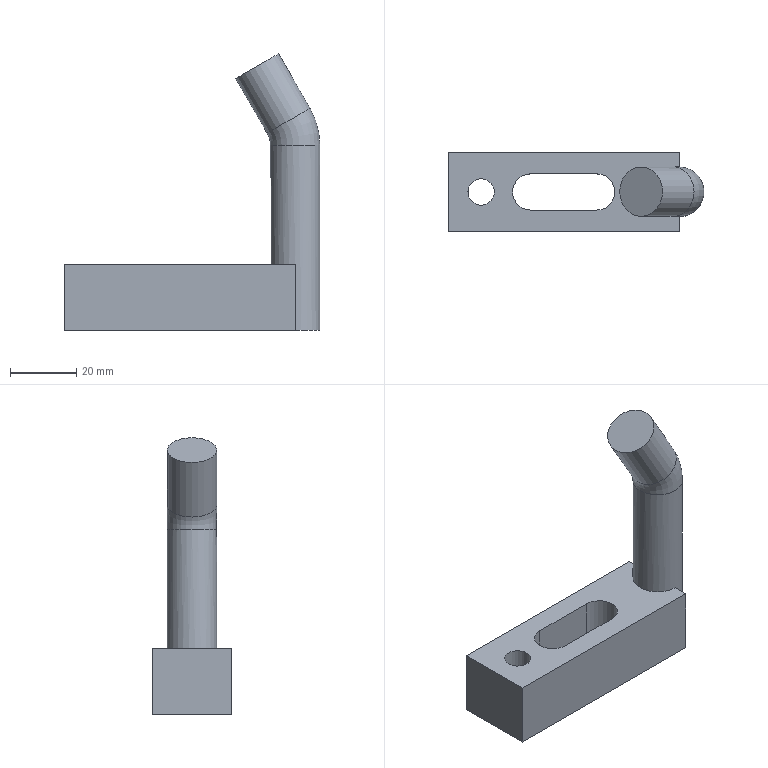Part | NX | features solid 2 | 1 solid | 16 faces | box 77.5 x 24 x 83.75 mm | volume 39178 mm3 | plane 10 | cylinder 5 | torus 1 | commonest cylinder face diameters 11 x2 15 x2 8 x1
STEP:
#1=CARTESIAN_POINT('',(-857.,457.5,-40.));
#2=VERTEX_POINT('',#1);
#3=CARTESIAN_POINT('',(-857.,457.5,-20.));
#4=VERTEX_POINT('',#3);
#5=CARTESIAN_POINT('',(-857.,457.5,15.981));
#6=DIRECTION('',(0.,0.,-1.));
#7=VECTOR('',#6,1000.);
#8=LINE('',#5,#7);
#9=EDGE_CURVE('',#2,#4,#8,.F.);
#10=ORIENTED_EDGE('',*,*,#9,.F.);
#11=CARTESIAN_POINT('',(-857.,462.,-40.));
#12=VERTEX_POINT('',#11);
#13=CARTESIAN_POINT('',(-857.,438.,-40.));
#14=DIRECTION('',(0.,1.,0.));
#15=VECTOR('',#14,1000.);
#16=LINE('',#13,#15);
#17=EDGE_CURVE('',#2,#12,#16,.T.);
#18=ORIENTED_EDGE('',*,*,#17,.T.);
#19=CARTESIAN_POINT('',(-857.,462.,-20.));
#20=VERTEX_POINT('',#19);
#21=CARTESIAN_POINT('',(-857.,462.,-20.));
#22=DIRECTION('',(0.,0.,-1.));
#23=VECTOR('',#22,1000.);
#24=LINE('',#21,#23);
#25=EDGE_CURVE('',#20,#12,#24,.T.);
#26=ORIENTED_EDGE('',*,*,#25,.F.);
#27=CARTESIAN_POINT('',(-857.,438.,-20.));
#28=DIRECTION('',(0.,1.,0.));
#29=VECTOR('',#28,1000.);
#30=LINE('',#27,#29);
#31=EDGE_CURVE('',#4,#20,#30,.T.);
#32=ORIENTED_EDGE('',*,*,#31,.F.);
#33=EDGE_LOOP('',(#10,#18,#26,#32));
#34=FACE_BOUND('',#33,.T.);
#35=CARTESIAN_POINT('',(-857.,438.,-20.));
#36=DIRECTION('',(-1.,0.,0.));
#37=DIRECTION('',(0.,0.,-1.));
#38=AXIS2_PLACEMENT_3D('',#35,#36,#37);
#39=PLANE('',#38);
#40=ADVANCED_FACE('',(#34),#39,.F.);
#41=CARTESIAN_POINT('',(-857.,442.5,-20.));
#42=VERTEX_POINT('',#41);
#43=CARTESIAN_POINT('',(-857.,442.5,-40.));
#44=VERTEX_POINT('',#43);
#45=CARTESIAN_POINT('',(-857.,442.5,15.981));
#46=DIRECTION('',(0.,0.,-1.));
#47=VECTOR('',#46,1000.);
#48=LINE('',#45,#47);
#49=EDGE_CURVE('',#42,#44,#48,.T.);
#50=ORIENTED_EDGE('',*,*,#49,.F.);
#51=CARTESIAN_POINT('',(-857.,438.,-20.));
#52=VERTEX_POINT('',#51);
#53=CARTESIAN_POINT('',(-857.,438.,-20.));
#54=DIRECTION('',(0.,1.,0.));
#55=VECTOR('',#54,1000.);
#56=LINE('',#53,#55);
#57=EDGE_CURVE('',#52,#42,#56,.T.);
#58=ORIENTED_EDGE('',*,*,#57,.F.);
#59=CARTESIAN_POINT('',(-857.,438.,-40.));
#60=VERTEX_POINT('',#59);
#61=CARTESIAN_POINT('',(-857.,438.,-20.));
#62=DIRECTION('',(0.,0.,-1.));
#63=VECTOR('',#62,1000.);
#64=LINE('',#61,#63);
#65=EDGE_CURVE('',#52,#60,#64,.T.);
#66=ORIENTED_EDGE('',*,*,#65,.T.);
#67=CARTESIAN_POINT('',(-857.,438.,-40.));
#68=DIRECTION('',(0.,1.,0.));
#69=VECTOR('',#68,1000.);
#70=LINE('',#67,#69);
#71=EDGE_CURVE('',#60,#44,#70,.T.);
#72=ORIENTED_EDGE('',*,*,#71,.T.);
#73=EDGE_LOOP('',(#50,#58,#66,#72));
#74=FACE_BOUND('',#73,.T.);
#75=CARTESIAN_POINT('',(-857.,438.,-20.));
#76=DIRECTION('',(-1.,0.,0.));
#77=DIRECTION('',(0.,0.,-1.));
#78=AXIS2_PLACEMENT_3D('',#75,#76,#77);
#79=PLANE('',#78);
#80=ADVANCED_FACE('',(#74),#79,.F.);
#81=CARTESIAN_POINT('',(-882.,444.5,-20.));
#82=VERTEX_POINT('',#81);
#83=CARTESIAN_POINT('',(-902.,444.5,-20.));
#84=VERTEX_POINT('',#83);
#85=CARTESIAN_POINT('',(-892.,444.5,-20.));
#86=DIRECTION('',(-1.,0.,0.));
#87=VECTOR('',#86,1000.);
#88=LINE('',#85,#87);
#89=EDGE_CURVE('',#82,#84,#88,.T.);
#90=ORIENTED_EDGE('',*,*,#89,.T.);
#91=CARTESIAN_POINT('',(-902.,455.5,-20.));
#92=VERTEX_POINT('',#91);
#93=CARTESIAN_POINT('',(-902.,450.,-20.));
#94=DIRECTION('',(0.,0.,1.));
#95=DIRECTION('',(-1.,0.,0.));
#96=AXIS2_PLACEMENT_3D('',#93,#94,#95);
#97=CIRCLE('',#96,5.5);
#98=EDGE_CURVE('',#92,#84,#97,.T.);
#99=ORIENTED_EDGE('',*,*,#98,.F.);
#100=CARTESIAN_POINT('',(-882.,455.5,-20.));
#101=VERTEX_POINT('',#100);
#102=CARTESIAN_POINT('',(-892.,455.5,-20.));
#103=DIRECTION('',(-1.,0.,0.));
#104=VECTOR('',#103,1000.);
#105=LINE('',#102,#104);
#106=EDGE_CURVE('',#101,#92,#105,.T.);
#107=ORIENTED_EDGE('',*,*,#106,.F.);
#108=CARTESIAN_POINT('',(-882.,450.,-20.));
#109=DIRECTION('',(0.,0.,1.));
#110=DIRECTION('',(-1.,0.,0.));
#111=AXIS2_PLACEMENT_3D('',#108,#109,#110);
#112=CIRCLE('',#111,5.5);
#113=EDGE_CURVE('',#82,#101,#112,.T.);
#114=ORIENTED_EDGE('',*,*,#113,.F.);
#115=EDGE_LOOP('',(#90,#99,#107,#114));
#116=FACE_BOUND('',#115,.T.);
#117=CARTESIAN_POINT('',(-913.,450.,-20.));
#118=VERTEX_POINT('',#117);
#119=CARTESIAN_POINT('',(-917.,450.,-20.));
#120=DIRECTION('',(0.,0.,-1.));
#121=DIRECTION('',(1.,0.,0.));
#122=AXIS2_PLACEMENT_3D('',#119,#120,#121);
#123=CIRCLE('',#122,4.);
#124=EDGE_CURVE('',#118,#118,#123,.T.);
#125=ORIENTED_EDGE('',*,*,#124,.T.);
#126=EDGE_LOOP('',(#125));
#127=FACE_BOUND('',#126,.T.);
#128=ORIENTED_EDGE('',*,*,#57,.T.);
#129=CARTESIAN_POINT('',(-857.,450.,-20.));
#130=DIRECTION('',(0.,0.,1.));
#131=DIRECTION('',(-1.,0.,0.));
#132=AXIS2_PLACEMENT_3D('',#129,#130,#131);
#133=CIRCLE('',#132,7.5);
#134=EDGE_CURVE('',#42,#4,#133,.F.);
#135=ORIENTED_EDGE('',*,*,#134,.T.);
#136=ORIENTED_EDGE('',*,*,#31,.T.);
#137=CARTESIAN_POINT('',(-927.,462.,-20.));
#138=VERTEX_POINT('',#137);
#139=CARTESIAN_POINT('',(-857.,462.,-20.));
#140=DIRECTION('',(-1.,0.,0.));
#141=VECTOR('',#140,1000.);
#142=LINE('',#139,#141);
#143=EDGE_CURVE('',#20,#138,#142,.T.);
#144=ORIENTED_EDGE('',*,*,#143,.T.);
#145=CARTESIAN_POINT('',(-927.,438.,-20.));
#146=VERTEX_POINT('',#145);
#147=CARTESIAN_POINT('',(-927.,462.,-20.));
#148=DIRECTION('',(0.,-1.,0.));
#149=VECTOR('',#148,1000.);
#150=LINE('',#147,#149);
#151=EDGE_CURVE('',#138,#146,#150,.T.);
#152=ORIENTED_EDGE('',*,*,#151,.T.);
#153=CARTESIAN_POINT('',(-927.,438.,-20.));
#154=DIRECTION('',(1.,0.,0.));
#155=VECTOR('',#154,1000.);
#156=LINE('',#153,#155);
#157=EDGE_CURVE('',#146,#52,#156,.T.);
#158=ORIENTED_EDGE('',*,*,#157,.T.);
#159=EDGE_LOOP('',(#128,#135,#136,#144,#152,#158));
#160=FACE_BOUND('',#159,.T.);
#161=CARTESIAN_POINT('',(-927.,438.,-20.));
#162=DIRECTION('',(0.,0.,1.));
#163=DIRECTION('',(-1.,0.,0.));
#164=AXIS2_PLACEMENT_3D('',#161,#162,#163);
#165=PLANE('',#164);
#166=ADVANCED_FACE('',(#116,#127,#160),#165,.T.);
#167=CARTESIAN_POINT('',(-927.,462.,-40.));
#168=VERTEX_POINT('',#167);
#169=CARTESIAN_POINT('',(-927.,438.,-40.));
#170=VERTEX_POINT('',#169);
#171=CARTESIAN_POINT('',(-927.,462.,-40.));
#172=DIRECTION('',(0.,-1.,0.));
#173=VECTOR('',#172,1000.);
#174=LINE('',#171,#173);
#175=EDGE_CURVE('',#168,#170,#174,.T.);
#176=ORIENTED_EDGE('',*,*,#175,.T.);
#177=CARTESIAN_POINT('',(-927.,438.,-20.));
#178=DIRECTION('',(0.,0.,-1.));
#179=VECTOR('',#178,1000.);
#180=LINE('',#177,#179);
#181=EDGE_CURVE('',#146,#170,#180,.T.);
#182=ORIENTED_EDGE('',*,*,#181,.F.);
#183=ORIENTED_EDGE('',*,*,#151,.F.);
#184=CARTESIAN_POINT('',(-927.,462.,-20.));
#185=DIRECTION('',(0.,0.,-1.));
#186=VECTOR('',#185,1000.);
#187=LINE('',#184,#186);
#188=EDGE_CURVE('',#138,#168,#187,.T.);
#189=ORIENTED_EDGE('',*,*,#188,.T.);
#190=EDGE_LOOP('',(#176,#182,#183,#189));
#191=FACE_BOUND('',#190,.T.);
#192=CARTESIAN_POINT('',(-927.,462.,-20.));
#193=DIRECTION('',(1.,0.,0.));
#194=DIRECTION('',(0.,0.,1.));
#195=AXIS2_PLACEMENT_3D('',#192,#193,#194);
#196=PLANE('',#195);
#197=ADVANCED_FACE('',(#191),#196,.F.);
#198=CARTESIAN_POINT('',(-927.,438.,-40.));
#199=DIRECTION('',(1.,0.,0.));
#200=VECTOR('',#199,1000.);
#201=LINE('',#198,#200);
#202=EDGE_CURVE('',#170,#60,#201,.T.);
#203=ORIENTED_EDGE('',*,*,#202,.T.);
#204=ORIENTED_EDGE('',*,*,#65,.F.);
#205=ORIENTED_EDGE('',*,*,#157,.F.);
#206=ORIENTED_EDGE('',*,*,#181,.T.);
#207=EDGE_LOOP('',(#203,#204,#205,#206));
#208=FACE_BOUND('',#207,.T.);
#209=CARTESIAN_POINT('',(-927.,438.,-20.));
#210=DIRECTION('',(0.,1.,0.));
#211=DIRECTION('',(-1.,0.,0.));
#212=AXIS2_PLACEMENT_3D('',#209,#210,#211);
#213=PLANE('',#212);
#214=ADVANCED_FACE('',(#208),#213,.F.);
#215=CARTESIAN_POINT('',(-857.,462.,-40.));
#216=DIRECTION('',(-1.,0.,0.));
#217=VECTOR('',#216,1000.);
#218=LINE('',#215,#217);
#219=EDGE_CURVE('',#12,#168,#218,.T.);
#220=ORIENTED_EDGE('',*,*,#219,.T.);
#221=ORIENTED_EDGE('',*,*,#188,.F.);
#222=ORIENTED_EDGE('',*,*,#143,.F.);
#223=ORIENTED_EDGE('',*,*,#25,.T.);
#224=EDGE_LOOP('',(#220,#221,#222,#223));
#225=FACE_BOUND('',#224,.T.);
#226=CARTESIAN_POINT('',(-857.,462.,-20.));
#227=DIRECTION('',(0.,-1.,0.));
#228=DIRECTION('',(1.,0.,0.));
#229=AXIS2_PLACEMENT_3D('',#226,#227,#228);
#230=PLANE('',#229);
#231=ADVANCED_FACE('',(#225),#230,.F.);
#232=ORIENTED_EDGE('',*,*,#17,.F.);
#233=CARTESIAN_POINT('',(-857.,450.,-40.));
#234=DIRECTION('',(0.,0.,1.));
#235=DIRECTION('',(-1.,0.,0.));
#236=AXIS2_PLACEMENT_3D('',#233,#234,#235);
#237=CIRCLE('',#236,7.5);
#238=EDGE_CURVE('',#44,#2,#237,.T.);
#239=ORIENTED_EDGE('',*,*,#238,.F.);
#240=ORIENTED_EDGE('',*,*,#71,.F.);
#241=ORIENTED_EDGE('',*,*,#202,.F.);
#242=ORIENTED_EDGE('',*,*,#175,.F.);
#243=ORIENTED_EDGE('',*,*,#219,.F.);
#244=EDGE_LOOP('',(#232,#239,#240,#241,#242,#243));
#245=FACE_BOUND('',#244,.T.);
#246=CARTESIAN_POINT('',(-902.,455.5,-40.));
#247=VERTEX_POINT('',#246);
#248=CARTESIAN_POINT('',(-902.,444.5,-40.));
#249=VERTEX_POINT('',#248);
#250=CARTESIAN_POINT('',(-902.,450.,-40.));
#251=DIRECTION('',(0.,0.,1.));
#252=DIRECTION('',(-1.,0.,0.));
#253=AXIS2_PLACEMENT_3D('',#250,#251,#252);
#254=CIRCLE('',#253,5.5);
#255=EDGE_CURVE('',#247,#249,#254,.T.);
#256=ORIENTED_EDGE('',*,*,#255,.T.);
#257=CARTESIAN_POINT('',(-882.,444.5,-40.));
#258=VERTEX_POINT('',#257);
#259=CARTESIAN_POINT('',(-882.,444.5,-40.));
#260=DIRECTION('',(-1.,0.,0.));
#261=VECTOR('',#260,1000.);
#262=LINE('',#259,#261);
#263=EDGE_CURVE('',#258,#249,#262,.T.);
#264=ORIENTED_EDGE('',*,*,#263,.F.);
#265=CARTESIAN_POINT('',(-882.,455.5,-40.));
#266=VERTEX_POINT('',#265);
#267=CARTESIAN_POINT('',(-882.,450.,-40.));
#268=DIRECTION('',(0.,0.,1.));
#269=DIRECTION('',(-1.,0.,0.));
#270=AXIS2_PLACEMENT_3D('',#267,#268,#269);
#271=CIRCLE('',#270,5.5);
#272=EDGE_CURVE('',#258,#266,#271,.T.);
#273=ORIENTED_EDGE('',*,*,#272,.T.);
#274=CARTESIAN_POINT('',(-882.,455.5,-40.));
#275=DIRECTION('',(-1.,0.,0.));
#276=VECTOR('',#275,1000.);
#277=LINE('',#274,#276);
#278=EDGE_CURVE('',#266,#247,#277,.T.);
#279=ORIENTED_EDGE('',*,*,#278,.T.);
#280=EDGE_LOOP('',(#256,#264,#273,#279));
#281=FACE_BOUND('',#280,.T.);
#282=CARTESIAN_POINT('',(-921.,450.,-40.));
#283=VERTEX_POINT('',#282);
#284=CARTESIAN_POINT('',(-917.,450.,-40.));
#285=DIRECTION('',(0.,0.,1.));
#286=DIRECTION('',(-1.,0.,0.));
#287=AXIS2_PLACEMENT_3D('',#284,#285,#286);
#288=CIRCLE('',#287,4.);
#289=EDGE_CURVE('',#283,#283,#288,.T.);
#290=ORIENTED_EDGE('',*,*,#289,.T.);
#291=EDGE_LOOP('',(#290));
#292=FACE_BOUND('',#291,.T.);
#293=CARTESIAN_POINT('',(-927.,438.,-40.));
#294=DIRECTION('',(0.,0.,1.));
#295=DIRECTION('',(-1.,0.,0.));
#296=AXIS2_PLACEMENT_3D('',#293,#294,#295);
#297=PLANE('',#296);
#298=ADVANCED_FACE('',(#245,#281,#292),#297,.F.);
#299=ORIENTED_EDGE('',*,*,#89,.F.);
#300=CARTESIAN_POINT('',(-882.,444.5,-20.));
#301=DIRECTION('',(0.,0.,1.));
#302=VECTOR('',#301,1000.);
#303=LINE('',#300,#302);
#304=EDGE_CURVE('',#258,#82,#303,.T.);
#305=ORIENTED_EDGE('',*,*,#304,.F.);
#306=ORIENTED_EDGE('',*,*,#263,.T.);
#307=CARTESIAN_POINT('',(-902.,444.5,-20.));
#308=DIRECTION('',(0.,0.,1.));
#309=VECTOR('',#308,1000.);
#310=LINE('',#307,#309);
#311=EDGE_CURVE('',#249,#84,#310,.T.);
#312=ORIENTED_EDGE('',*,*,#311,.T.);
#313=EDGE_LOOP('',(#299,#305,#306,#312));
#314=FACE_BOUND('',#313,.T.);
#315=CARTESIAN_POINT('',(-892.,444.5,-20.));
#316=DIRECTION('',(0.,-1.,0.));
#317=DIRECTION('',(0.,0.,1.));
#318=AXIS2_PLACEMENT_3D('',#315,#316,#317);
#319=PLANE('',#318);
#320=ADVANCED_FACE('',(#314),#319,.F.);
#321=ORIENTED_EDGE('',*,*,#113,.T.);
#322=CARTESIAN_POINT('',(-882.,455.5,-20.));
#323=DIRECTION('',(0.,0.,1.));
#324=VECTOR('',#323,1000.);
#325=LINE('',#322,#324);
#326=EDGE_CURVE('',#266,#101,#325,.T.);
#327=ORIENTED_EDGE('',*,*,#326,.F.);
#328=ORIENTED_EDGE('',*,*,#272,.F.);
#329=ORIENTED_EDGE('',*,*,#304,.T.);
#330=EDGE_LOOP('',(#321,#327,#328,#329));
#331=FACE_BOUND('',#330,.T.);
#332=CARTESIAN_POINT('',(-882.,450.,-20.));
#333=DIRECTION('',(0.,0.,1.));
#334=DIRECTION('',(-1.,0.,0.));
#335=AXIS2_PLACEMENT_3D('',#332,#333,#334);
#336=CYLINDRICAL_SURFACE('',#335,5.5);
#337=ADVANCED_FACE('',(#331),#336,.F.);
#338=ORIENTED_EDGE('',*,*,#106,.T.);
#339=CARTESIAN_POINT('',(-902.,455.5,-20.));
#340=DIRECTION('',(0.,0.,1.));
#341=VECTOR('',#340,1000.);
#342=LINE('',#339,#341);
#343=EDGE_CURVE('',#247,#92,#342,.T.);
#344=ORIENTED_EDGE('',*,*,#343,.F.);
#345=ORIENTED_EDGE('',*,*,#278,.F.);
#346=ORIENTED_EDGE('',*,*,#326,.T.);
#347=EDGE_LOOP('',(#338,#344,#345,#346));
#348=FACE_BOUND('',#347,.T.);
#349=CARTESIAN_POINT('',(-892.,455.5,-20.));
#350=DIRECTION('',(0.,1.,0.));
#351=DIRECTION('',(0.,0.,-1.));
#352=AXIS2_PLACEMENT_3D('',#349,#350,#351);
#353=PLANE('',#352);
#354=ADVANCED_FACE('',(#348),#353,.F.);
#355=ORIENTED_EDGE('',*,*,#98,.T.);
#356=ORIENTED_EDGE('',*,*,#311,.F.);
#357=ORIENTED_EDGE('',*,*,#255,.F.);
#358=ORIENTED_EDGE('',*,*,#343,.T.);
#359=EDGE_LOOP('',(#355,#356,#357,#358));
#360=FACE_BOUND('',#359,.T.);
#361=CARTESIAN_POINT('',(-902.,450.,-20.));
#362=DIRECTION('',(0.,0.,1.));
#363=DIRECTION('',(-1.,0.,0.));
#364=AXIS2_PLACEMENT_3D('',#361,#362,#363);
#365=CYLINDRICAL_SURFACE('',#364,5.5);
#366=ADVANCED_FACE('',(#360),#365,.F.);
#367=ORIENTED_EDGE('',*,*,#124,.F.);
#368=EDGE_LOOP('',(#367));
#369=FACE_BOUND('',#368,.T.);
#370=ORIENTED_EDGE('',*,*,#289,.F.);
#371=EDGE_LOOP('',(#370));
#372=FACE_BOUND('',#371,.T.);
#373=CARTESIAN_POINT('',(-917.,450.,-20.));
#374=DIRECTION('',(0.,0.,-1.));
#375=DIRECTION('',(1.,0.,0.));
#376=AXIS2_PLACEMENT_3D('',#373,#374,#375);
#377=CYLINDRICAL_SURFACE('',#376,4.);
#378=ADVANCED_FACE('',(#369,#372),#377,.F.);
#379=CARTESIAN_POINT('',(-864.5,450.,15.981));
#380=VERTEX_POINT('',#379);
#381=CARTESIAN_POINT('',(-857.,450.,15.981));
#382=DIRECTION('',(0.,0.,1.));
#383=DIRECTION('',(-1.,0.,0.));
#384=AXIS2_PLACEMENT_3D('',#381,#382,#383);
#385=CIRCLE('',#384,7.5);
#386=EDGE_CURVE('',#380,#380,#385,.T.);
#387=ORIENTED_EDGE('',*,*,#386,.F.);
#388=EDGE_LOOP('',(#387));
#389=FACE_BOUND('',#388,.T.);
#390=ORIENTED_EDGE('',*,*,#238,.T.);
#391=ORIENTED_EDGE('',*,*,#9,.T.);
#392=ORIENTED_EDGE('',*,*,#134,.F.);
#393=ORIENTED_EDGE('',*,*,#49,.T.);
#394=EDGE_LOOP('',(#390,#391,#392,#393));
#395=FACE_BOUND('',#394,.T.);
#396=CARTESIAN_POINT('',(-857.,450.,15.981));
#397=DIRECTION('',(0.,0.,-1.));
#398=DIRECTION('',(1.,0.,0.));
#399=AXIS2_PLACEMENT_3D('',#396,#397,#398);
#400=CYLINDRICAL_SURFACE('',#399,7.5);
#401=ADVANCED_FACE('',(#389,#395),#400,.T.);
#402=CARTESIAN_POINT('',(-865.505,450.,19.731));
#403=VERTEX_POINT('',#402);
#404=CARTESIAN_POINT('',(-859.01,450.,23.481));
#405=DIRECTION('',(-0.5,0.,0.866));
#406=DIRECTION('',(-0.866,0.,-0.5));
#407=AXIS2_PLACEMENT_3D('',#404,#405,#406);
#408=CIRCLE('',#407,7.5);
#409=EDGE_CURVE('',#403,#403,#408,.T.);
#410=ORIENTED_EDGE('',*,*,#409,.T.);
#411=EDGE_LOOP('',(#410));
#412=FACE_BOUND('',#411,.T.);
#413=CARTESIAN_POINT('',(-875.042,450.,36.25));
#414=VERTEX_POINT('',#413);
#415=CARTESIAN_POINT('',(-868.547,450.,40.));
#416=DIRECTION('',(-0.5,0.,0.866));
#417=DIRECTION('',(-0.866,0.,-0.5));
#418=AXIS2_PLACEMENT_3D('',#415,#416,#417);
#419=CIRCLE('',#418,7.5);
#420=EDGE_CURVE('',#414,#414,#419,.T.);
#421=ORIENTED_EDGE('',*,*,#420,.F.);
#422=EDGE_LOOP('',(#421));
#423=FACE_BOUND('',#422,.T.);
#424=CARTESIAN_POINT('',(-859.01,450.,23.481));
#425=DIRECTION('',(-0.5,0.,0.866));
#426=DIRECTION('',(-0.866,0.,-0.5));
#427=AXIS2_PLACEMENT_3D('',#424,#425,#426);
#428=CYLINDRICAL_SURFACE('',#427,7.5);
#429=ADVANCED_FACE('',(#412,#423),#428,.T.);
#430=ORIENTED_EDGE('',*,*,#386,.T.);
#431=EDGE_LOOP('',(#430));
#432=FACE_BOUND('',#431,.T.);
#433=ORIENTED_EDGE('',*,*,#409,.F.);
#434=EDGE_LOOP('',(#433));
#435=FACE_BOUND('',#434,.T.);
#436=CARTESIAN_POINT('',(-872.,450.,15.981));
#437=DIRECTION('',(0.,-1.,0.));
#438=DIRECTION('',(0.,0.,1.));
#439=AXIS2_PLACEMENT_3D('',#436,#437,#438);
#440=TOROIDAL_SURFACE('',#439,15.,7.5);
#441=ADVANCED_FACE('',(#432,#435),#440,.T.);
#442=ORIENTED_EDGE('',*,*,#420,.T.);
#443=EDGE_LOOP('',(#442));
#444=FACE_BOUND('',#443,.T.);
#445=CARTESIAN_POINT('',(-868.547,450.,40.));
#446=DIRECTION('',(-0.5,0.,0.866));
#447=DIRECTION('',(-0.866,0.,-0.5));
#448=AXIS2_PLACEMENT_3D('',#445,#446,#447);
#449=PLANE('',#448);
#450=ADVANCED_FACE('',(#444),#449,.T.);
#451=CLOSED_SHELL('',(#40,#80,#166,#197,#214,#231,#298,#320,#337,#354,#366,#378,#401,#429,#441,#450));
#452=MANIFOLD_SOLID_BREP('',#451);
#453=(LENGTH_UNIT()NAMED_UNIT(*)SI_UNIT(.MILLI.,.METRE.));
#454=UNCERTAINTY_MEASURE_WITH_UNIT(LENGTH_MEASURE(0.00001),#453,'','');
#455=(NAMED_UNIT(*)PLANE_ANGLE_UNIT()SI_UNIT($,.RADIAN.));
#456=(NAMED_UNIT(*)SI_UNIT($,.STERADIAN.)SOLID_ANGLE_UNIT());
#457=(GEOMETRIC_REPRESENTATION_CONTEXT(3)GLOBAL_UNCERTAINTY_ASSIGNED_CONTEXT((#454))GLOBAL_UNIT_ASSIGNED_CONTEXT((#453,#455,#456))REPRESENTATION_CONTEXT('',''));
#458=ADVANCED_BREP_SHAPE_REPRESENTATION('',(#452),#457);